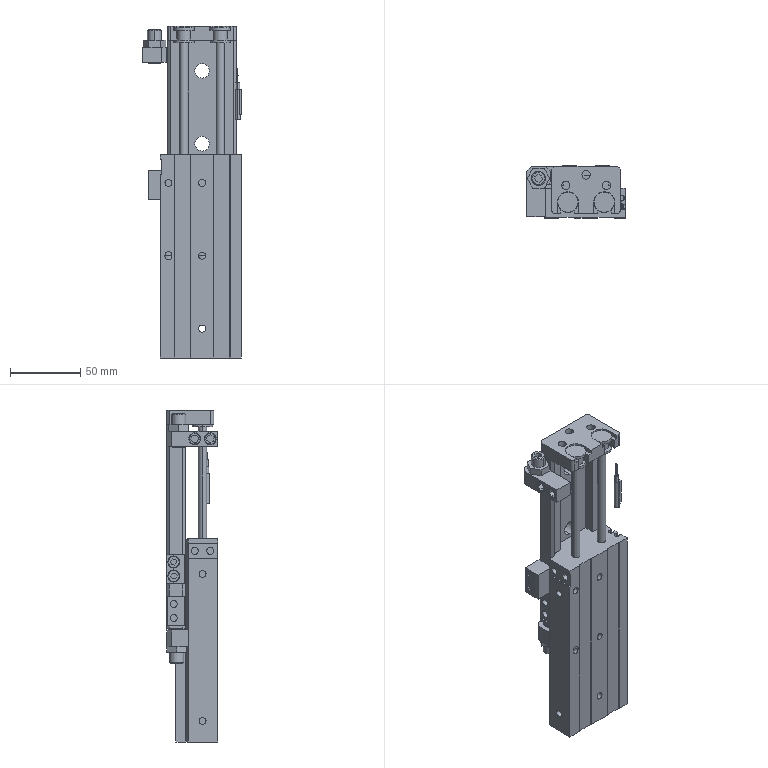Part | NX | 9 solids | 522 faces | box 70.6 x 37 x 237 mm | volume 281701 mm3 | plane 315 | cylinder 183 | cone 24 | commonest cylinder face diameters 5 x52 8.5 x16 6 x14 10 x11 0.5 x8 1 x8